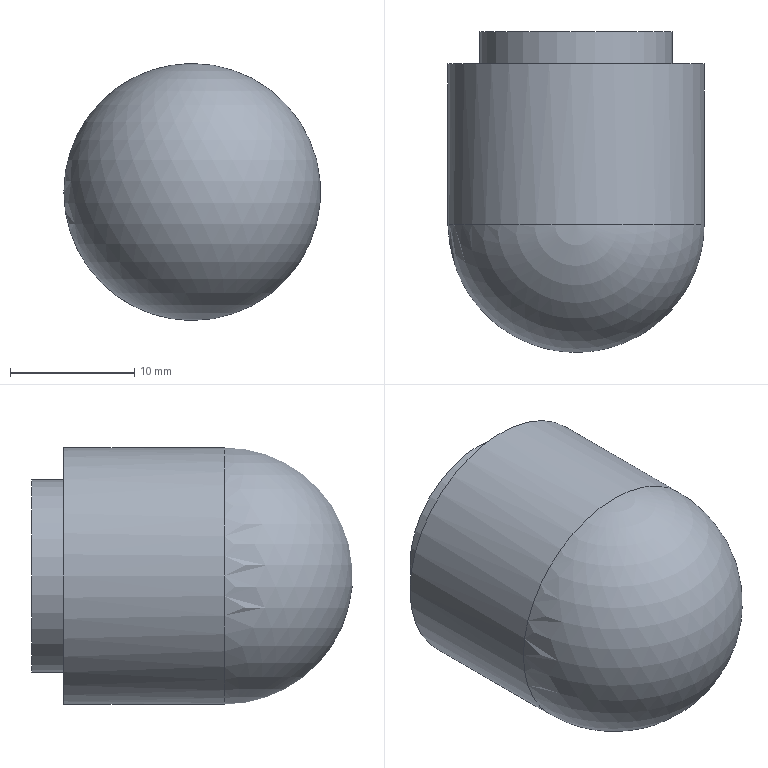Part | STEP file | basic_gh_motor_gh1_11 | 1 solid | 5 faces | box 20.64 x 25.8 x 20.64 mm | volume 7104 mm3 | cylinder 2 | plane 2 | sphere 1 | commonest cylinder face diameters 15.48 x1 20.64 x1
STEP:
#1=CARTESIAN_POINT('',(-181.73,29.93,87.25));
#2=VERTEX_POINT('',#1);
#3=CARTESIAN_POINT('',(-171.41,29.93,87.25));
#4=DIRECTION('',(0.,1.,0.));
#5=DIRECTION('',(1.,0.,0.));
#6=AXIS2_PLACEMENT_3D('',#3,#4,#5);
#7=CIRCLE('',#6,10.32);
#8=EDGE_CURVE('',#2,#2,#7,.T.);
#9=ORIENTED_EDGE('',*,*,#8,.F.);
#10=EDGE_LOOP('',(#9));
#11=FACE_OUTER_BOUND('',#10,.T.);
#12=CARTESIAN_POINT('',(-171.41,29.93,87.25));
#13=DIRECTION('',(0.,0.,1.));
#14=DIRECTION('',(0.,1.,0.));
#15=AXIS2_PLACEMENT_3D('',#12,#13,#14);
#16=SPHERICAL_SURFACE('',#15,10.32);
#17=ADVANCED_FACE('',(#11),#16,.T.);
#18=CARTESIAN_POINT('',(-181.73,42.83,87.25));
#19=VERTEX_POINT('',#18);
#20=CARTESIAN_POINT('',(-171.41,42.83,87.25));
#21=DIRECTION('',(0.,1.,0.));
#22=DIRECTION('',(1.,0.,0.));
#23=AXIS2_PLACEMENT_3D('',#20,#21,#22);
#24=CIRCLE('',#23,10.32);
#25=EDGE_CURVE('',#19,#19,#24,.T.);
#26=ORIENTED_EDGE('',*,*,#25,.F.);
#27=CARTESIAN_POINT('',(-181.73,36.38,87.25));
#28=DIRECTION('',(0.,-1.,0.));
#29=VECTOR('',#28,10.32);
#30=LINE('',#27,#29);
#31=EDGE_CURVE('',#19,#2,#30,.T.);
#32=ORIENTED_EDGE('',*,*,#31,.T.);
#33=ORIENTED_EDGE('',*,*,#8,.T.);
#34=ORIENTED_EDGE('',*,*,#31,.F.);
#35=EDGE_LOOP('',(#26,#32,#33,#34));
#36=FACE_OUTER_BOUND('',#35,.T.);
#37=CARTESIAN_POINT('',(-171.41,36.38,87.25));
#38=DIRECTION('',(0.,1.,0.));
#39=DIRECTION('',(1.,0.,0.));
#40=AXIS2_PLACEMENT_3D('',#37,#38,#39);
#41=CYLINDRICAL_SURFACE('',#40,10.32);
#42=ADVANCED_FACE('',(#36),#41,.T.);
#43=ORIENTED_EDGE('',*,*,#25,.T.);
#44=EDGE_LOOP('',(#43));
#45=FACE_OUTER_BOUND('',#44,.T.);
#46=CARTESIAN_POINT('',(-179.15,42.83,87.25));
#47=VERTEX_POINT('',#46);
#48=CARTESIAN_POINT('',(-171.41,42.83,87.25));
#49=DIRECTION('',(0.,1.,0.));
#50=DIRECTION('',(1.,0.,0.));
#51=AXIS2_PLACEMENT_3D('',#48,#49,#50);
#52=CIRCLE('',#51,7.74);
#53=EDGE_CURVE('',#47,#47,#52,.T.);
#54=ORIENTED_EDGE('',*,*,#53,.F.);
#55=EDGE_LOOP('',(#54));
#56=FACE_BOUND('',#55,.T.);
#57=CARTESIAN_POINT('',(-162.38,42.83,87.25));
#58=DIRECTION('',(0.,1.,0.));
#59=DIRECTION('',(1.,0.,0.));
#60=AXIS2_PLACEMENT_3D('',#57,#58,#59);
#61=PLANE('',#60);
#62=ADVANCED_FACE('',(#45,#56),#61,.T.);
#63=CARTESIAN_POINT('',(-179.15,45.41,87.25));
#64=VERTEX_POINT('',#63);
#65=CARTESIAN_POINT('',(-171.41,45.41,87.25));
#66=DIRECTION('',(0.,1.,0.));
#67=DIRECTION('',(1.,0.,0.));
#68=AXIS2_PLACEMENT_3D('',#65,#66,#67);
#69=CIRCLE('',#68,7.74);
#70=EDGE_CURVE('',#64,#64,#69,.T.);
#71=ORIENTED_EDGE('',*,*,#70,.F.);
#72=CARTESIAN_POINT('',(-179.15,44.12,87.25));
#73=DIRECTION('',(0.,-1.,0.));
#74=VECTOR('',#73,7.74);
#75=LINE('',#72,#74);
#76=EDGE_CURVE('',#64,#47,#75,.T.);
#77=ORIENTED_EDGE('',*,*,#76,.T.);
#78=ORIENTED_EDGE('',*,*,#53,.T.);
#79=ORIENTED_EDGE('',*,*,#76,.F.);
#80=EDGE_LOOP('',(#71,#77,#78,#79));
#81=FACE_OUTER_BOUND('',#80,.T.);
#82=CARTESIAN_POINT('',(-171.41,44.12,87.25));
#83=DIRECTION('',(0.,1.,0.));
#84=DIRECTION('',(1.,0.,0.));
#85=AXIS2_PLACEMENT_3D('',#82,#83,#84);
#86=CYLINDRICAL_SURFACE('',#85,7.74);
#87=ADVANCED_FACE('',(#81),#86,.T.);
#88=ORIENTED_EDGE('',*,*,#70,.T.);
#89=EDGE_LOOP('',(#88));
#90=FACE_OUTER_BOUND('',#89,.T.);
#91=CARTESIAN_POINT('',(-167.54,45.41,87.25));
#92=DIRECTION('',(0.,1.,0.));
#93=DIRECTION('',(1.,0.,0.));
#94=AXIS2_PLACEMENT_3D('',#91,#92,#93);
#95=PLANE('',#94);
#96=ADVANCED_FACE('',(#90),#95,.T.);
#97=CLOSED_SHELL('',(#17,#42,#62,#87,#96));
#98=MANIFOLD_SOLID_BREP('',#97);
#99=(LENGTH_UNIT()NAMED_UNIT(*)SI_UNIT(.MILLI.,.METRE.));
#100=UNCERTAINTY_MEASURE_WITH_UNIT(LENGTH_MEASURE(0.01),#99,'','');
#101=(NAMED_UNIT(*)PLANE_ANGLE_UNIT()SI_UNIT($,.RADIAN.));
#102=(NAMED_UNIT(*)SI_UNIT($,.STERADIAN.)SOLID_ANGLE_UNIT());
#103=(GEOMETRIC_REPRESENTATION_CONTEXT(3)GLOBAL_UNCERTAINTY_ASSIGNED_CONTEXT((#100))GLOBAL_UNIT_ASSIGNED_CONTEXT((#99,#101,#102))REPRESENTATION_CONTEXT('',''));
#104=ADVANCED_BREP_SHAPE_REPRESENTATION('',(#98),#103);